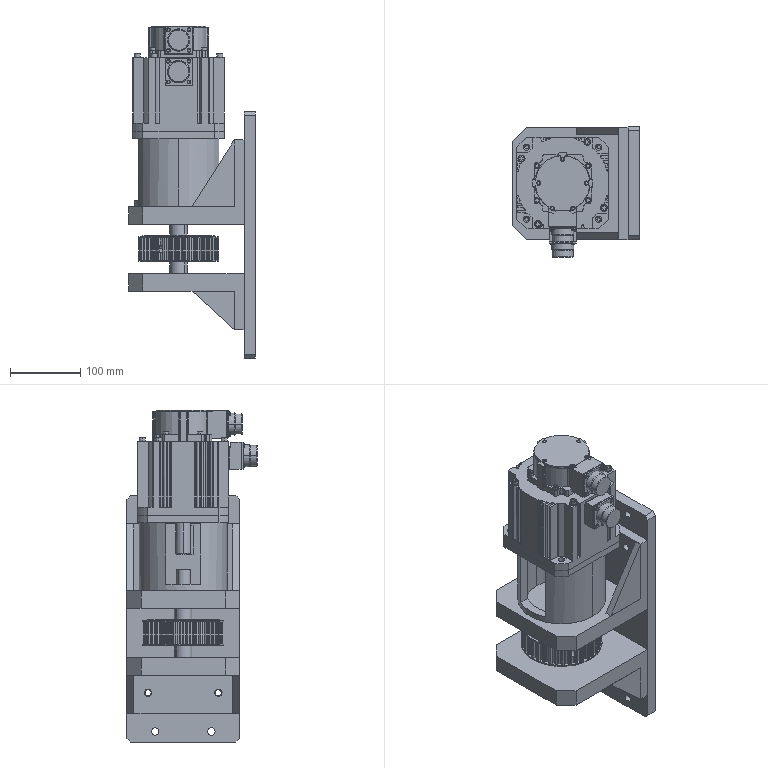Part | SolidWorks | features CompositeCurve 1 | 13 solids | 1233 faces | box 180 x 185 x 472 mm | volume 5233000 mm3 | cylinder 648 | plane 481 | cone 58 | spline 46 | commonest cylinder face diameters 1 x90 1.2 x89 1.6 x86 112.74 x36 2 x30 10.5 x24